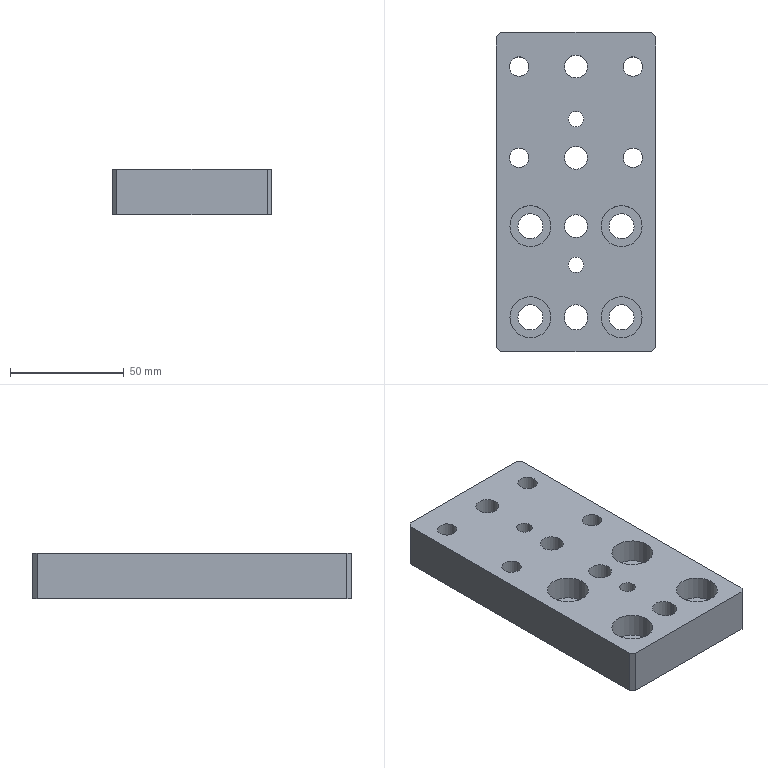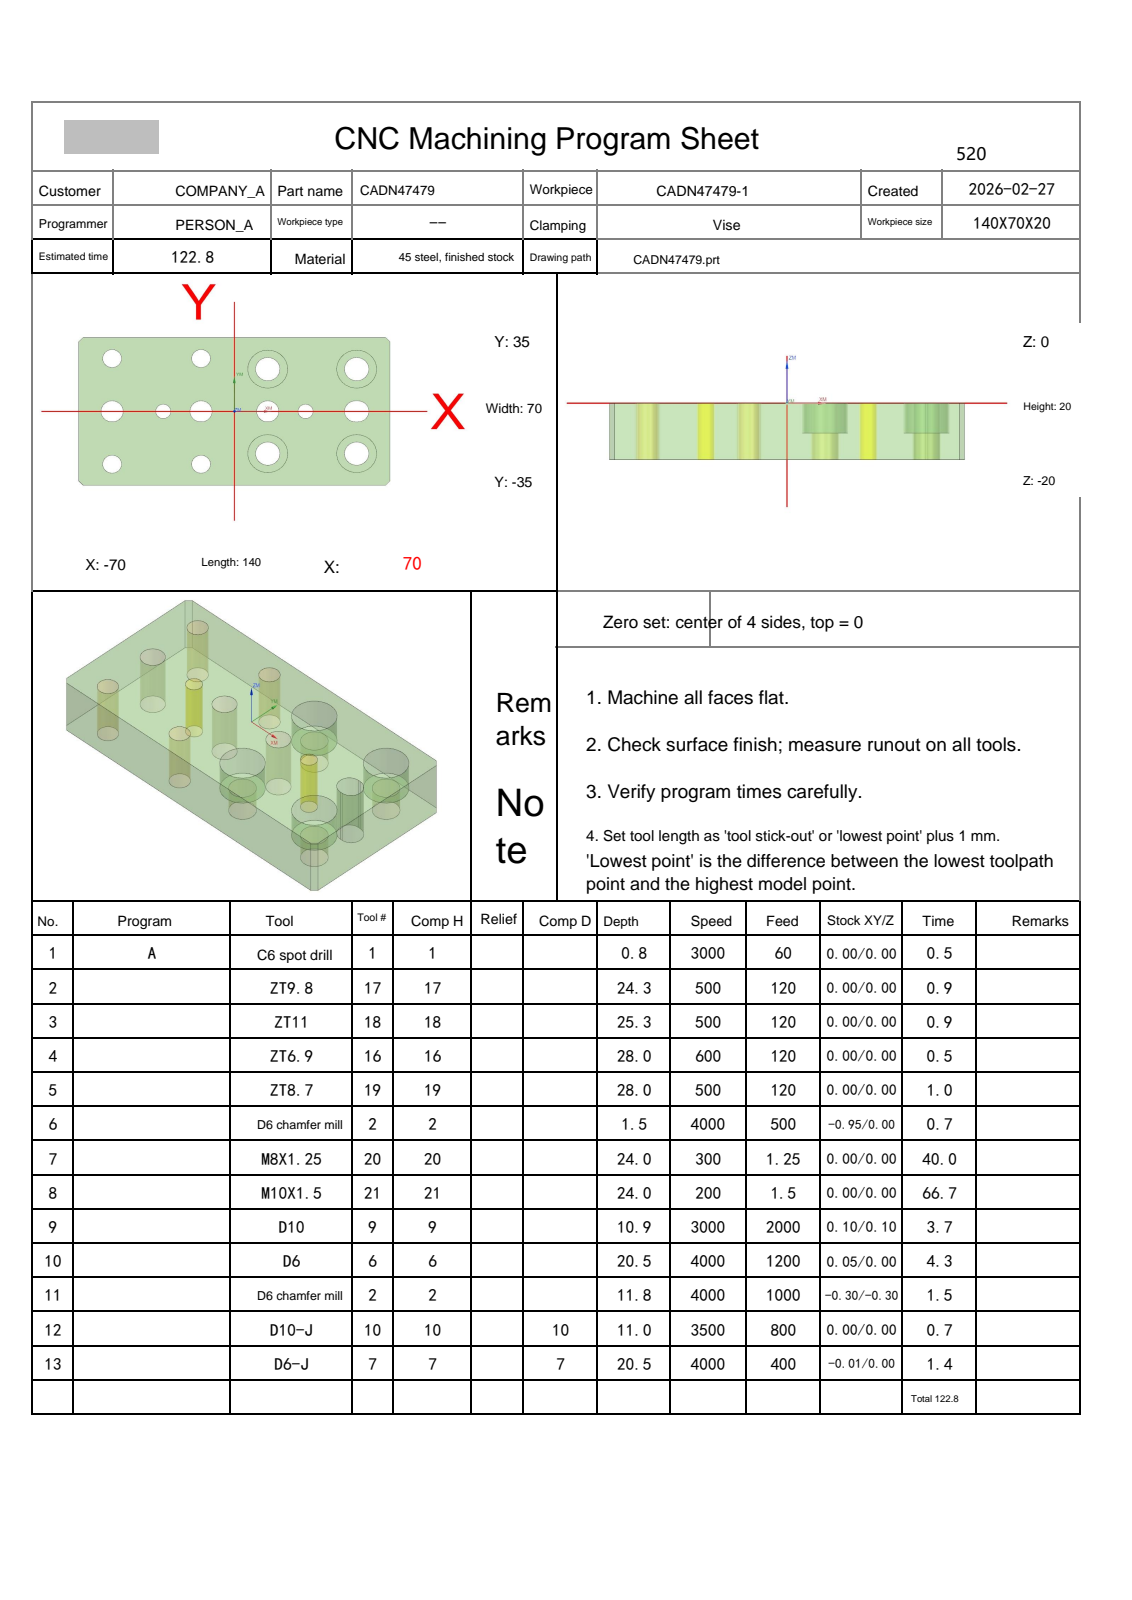NC program | NX | posted by the shop | part box 70 x 140 x 20 mm
Lines 3435 to 3634 of 3634:
N13 T07 M06
(D6-J  D=6. R=0. H=07 ce=-0.01 di=0.20)
G00 G90 G54 X-55. Y0.0 M03 S4000
G43 H07 Z30.
M08
Z.5
G41 D07
G01 X-54.804 Y.039 F400.
G03 X-54.005 Y1.015 I-.196 J.976
X-55. Y2.01 I-.995 J0.0
X-55. Y2.01 Z-1.5 I0.0 J-2.01
X-55. Y2.01 Z-3.5 I0.0 J-2.01
X-55. Y2.01 Z-5.5 I0.0 J-2.01
X-55. Y2.01 Z-7.5 I0.0 J-2.01
X-55. Y2.01 Z-9.5 I0.0 J-2.01
X-55. Y2.01 Z-11.5 I0.0 J-2.01
X-55. Y2.01 Z-13.5 I0.0 J-2.01
X-55. Y2.01 Z-15.5 I0.0 J-2.01
X-55. Y2.01 Z-17.5 I0.0 J-2.01
X-55. Y2.01 Z-19.5 I0.0 J-2.01
X-55. Y-2.01 Z-20.5 I0.0 J-2.01
X-52.99 Y0.0 I0.0 J2.01
X-55. Y2.01 I-2.01 J0.0
X-57.01 Y0.0 I0.0 J-2.01
X-55. Y-2.01 I2.01 J0.0
X-54.005 Y-1.015 I0.0 J.995
X-54.804 Y-.039 I-.995 J0.0
G01 G40 X-55. Y0.0
G00 Z30.
X-15.
Z.5
G41 D07
G01 X-14.804 Y.039
G03 X-14.005 Y1.015 I-.196 J.976
X-15. Y2.01 I-.995 J0.0
X-15. Y2.01 Z-1.5 I0.0 J-2.01
X-15. Y2.01 Z-3.5 I0.0 J-2.01
X-15. Y2.01 Z-5.5 I0.0 J-2.01
X-15. Y2.01 Z-7.5 I0.0 J-2.01
X-15. Y2.01 Z-9.5 I0.0 J-2.01
X-15. Y2.01 Z-11.5 I0.0 J-2.01
X-15. Y2.01 Z-13.5 I0.0 J-2.01
X-15. Y2.01 Z-15.5 I0.0 J-2.01
X-15. Y2.01 Z-17.5 I0.0 J-2.01
X-15. Y2.01 Z-19.5 I0.0 J-2.01
X-15. Y-2.01 Z-20.5 I0.0 J-2.01
X-12.99 Y0.0 I0.0 J2.01
X-15. Y2.01 I-2.01 J0.0
X-17.01 Y0.0 I0.0 J-2.01
X-15. Y-2.01 I2.01 J0.0
X-14.005 Y-1.015 I0.0 J.995
X-14.804 Y-.039 I-.995 J0.0
G01 G40 X-15. Y0.0
G00 Z30.
X15.
Z.5
G41 D07
G01 X15.196 Y.039
G03 X15.995 Y1.015 I-.196 J.976
X15. Y2.01 I-.995 J0.0
X15. Y2.01 Z-1.5 I0.0 J-2.01
X15. Y2.01 Z-3.5 I0.0 J-2.01
X15. Y2.01 Z-5.5 I0.0 J-2.01
X15. Y2.01 Z-7.5 I0.0 J-2.01
X15. Y2.01 Z-9.5 I0.0 J-2.01
X15. Y2.01 Z-11.5 I0.0 J-2.01
X15. Y2.01 Z-13.5 I0.0 J-2.01
X15. Y2.01 Z-15.5 I0.0 J-2.01
X15. Y2.01 Z-17.5 I0.0 J-2.01
X15. Y2.01 Z-19.5 I0.0 J-2.01
X15. Y-2.01 Z-20.5 I0.0 J-2.01
X17.01 Y0.0 I0.0 J2.01
X15. Y2.01 I-2.01 J0.0
X12.99 Y0.0 I0.0 J-2.01
X15. Y-2.01 I2.01 J0.0
X15.995 Y-1.015 I0.0 J.995
X15.196 Y-.039 I-.995 J0.0
G01 G40 X15. Y0.0
G00 Z30.
G00 G90 X54.8 Y-1.71 M03 S4000
Z30.
Z-2.883
G01 Z-3.383 F400.
G41 D07
Y-1.81
G03 X55. Y-2.01 I.2 J0.0
G01 X55.5
G03 X57.51 Y0.0 I0.0 J2.01
X55.5 Y2.01 I-2.01 J0.0
G01 X54.5
G03 X52.49 Y0.0 I0.0 J-2.01
X54.5 Y-2.01 I2.01 J0.0
G01 X55.
X55.5
G03 X55.7 Y-1.81 I0.0 J.2
G01 Y-1.799
G40 Y-1.699
Z-2.883
G00 Z.5
X54.8 Y-1.71
Z-6.267
G01 Z-6.767
G41 D07
Y-1.81
G03 X55. Y-2.01 I.2 J0.0
G01 X55.5
G03 X57.51 Y0.0 I0.0 J2.01
X55.5 Y2.01 I-2.01 J0.0
G01 X54.5
G03 X52.49 Y0.0 I0.0 J-2.01
X54.5 Y-2.01 I2.01 J0.0
G01 X55.
X55.5
G03 X55.7 Y-1.81 I0.0 J.2
G01 Y-1.799
G40 Y-1.699
Z-6.267
G00 Z-2.883
X54.8 Y-1.71
Z-9.65
G01 Z-10.15
G41 D07
Y-1.81
G03 X55. Y-2.01 I.2 J0.0
G01 X55.5
G03 X57.51 Y0.0 I0.0 J2.01
X55.5 Y2.01 I-2.01 J0.0
G01 X54.5
G03 X52.49 Y0.0 I0.0 J-2.01
X54.5 Y-2.01 I2.01 J0.0
G01 X55.
X55.5
G03 X55.7 Y-1.81 I0.0 J.2
G01 Y-1.799
G40 Y-1.699
Z-9.65
G00 Z-6.267
X54.8 Y-1.71
Z-13.033
G01 Z-13.533
G41 D07
Y-1.81
G03 X55. Y-2.01 I.2 J0.0
G01 X55.5
G03 X57.51 Y0.0 I0.0 J2.01
X55.5 Y2.01 I-2.01 J0.0
G01 X54.5
G03 X52.49 Y0.0 I0.0 J-2.01
X54.5 Y-2.01 I2.01 J0.0
G01 X55.
X55.5
G03 X55.7 Y-1.81 I0.0 J.2
G01 Y-1.799
G40 Y-1.699
Z-13.033
G00 Z-9.65
X54.8 Y-1.71
Z-16.417
G01 Z-16.917
G41 D07
Y-1.81
G03 X55. Y-2.01 I.2 J0.0
G01 X55.5
G03 X57.51 Y0.0 I0.0 J2.01
X55.5 Y2.01 I-2.01 J0.0
G01 X54.5
G03 X52.49 Y0.0 I0.0 J-2.01
X54.5 Y-2.01 I2.01 J0.0
G01 X55.
X55.5
G03 X55.7 Y-1.81 I0.0 J.2
G01 Y-1.799
G40 Y-1.699
Z-16.417
G00 Z-13.033
X54.8 Y-1.71
Z-19.8
G01 Z-20.3
G41 D07
Y-1.81
G03 X55. Y-2.01 I.2 J0.0
G01 X55.5
G03 X57.51 Y0.0 I0.0 J2.01
X55.5 Y2.01 I-2.01 J0.0
G01 X54.5
G03 X52.49 Y0.0 I0.0 J-2.01
X54.5 Y-2.01 I2.01 J0.0
G01 X55.
X55.5
G03 X55.7 Y-1.81 I0.0 J.2
G01 Y-1.799
G40 Y-1.699
Z-19.8
G00 Z30.
M05
M09
G91 G28 Z0.0
G91 G28 Y0.0
M30
%